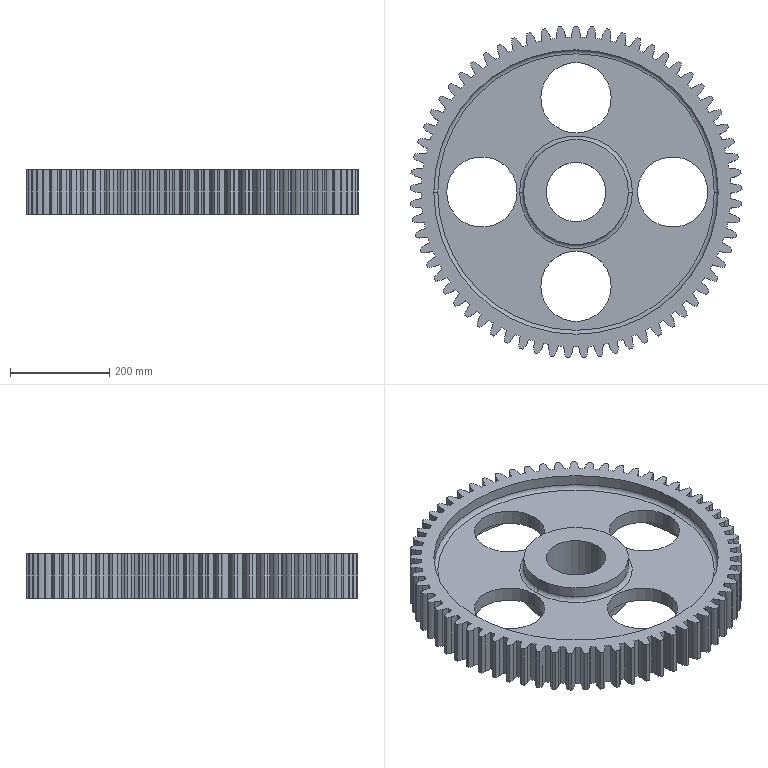Part | Creo | features PROTRUSION 66, CURVE 5, CUT 3, DATUM PLANE 3, COORDINATE SYSTEM 1, PATTERN 1, ROUND 1 | 1 solid | 422 faces | box 669.936 x 669.757 x 90 mm | volume 13299153 mm3 | cylinder 278 | plane 136 | torus 8 | commonest cylinder face diameters 50.73 x65 53.572 x65 625 x65 670 x65 142.063 x8 211.579 x4